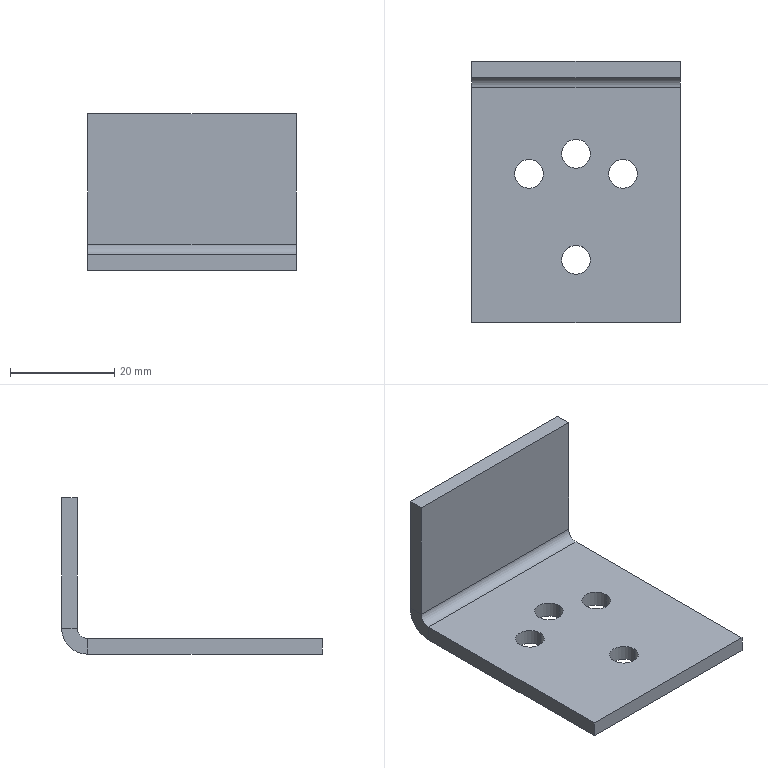Part | SolidWorks | features EdgeFlange 1, FlatPattern 1, HoleWzd 1, SMBaseFlange 1, SheetMetal 1 | 1 solid | 22 faces | box 40 x 50 x 30 mm | volume 8775 mm3 | plane 12 | cylinder 10 | commonest cylinder face diameters 5.5 x8 4 x1 10 x1
STEP:
#1=CARTESIAN_POINT('',(-11.75,3.5,-3.));
#2=VERTEX_POINT('',#1);
#3=CARTESIAN_POINT('',(-6.25,3.5,-3.));
#4=VERTEX_POINT('',#3);
#5=CARTESIAN_POINT('',(-9.,3.5,-3.));
#6=DIRECTION('',(0.,0.,1.));
#7=DIRECTION('',(1.,0.,0.));
#8=AXIS2_PLACEMENT_3D('',#5,#6,#7);
#9=CIRCLE('',#8,2.75);
#10=EDGE_CURVE('',#2,#4,#9,.T.);
#11=ORIENTED_EDGE('',*,*,#10,.F.);
#12=CARTESIAN_POINT('',(-11.75,3.5,0.));
#13=VERTEX_POINT('',#12);
#14=CARTESIAN_POINT('',(-11.75,3.5,0.));
#15=DIRECTION('',(0.,0.,1.));
#16=VECTOR('',#15,1000.);
#17=LINE('',#14,#16);
#18=EDGE_CURVE('',#2,#13,#17,.T.);
#19=ORIENTED_EDGE('',*,*,#18,.T.);
#20=CARTESIAN_POINT('',(-6.25,3.5,0.));
#21=VERTEX_POINT('',#20);
#22=CARTESIAN_POINT('',(-9.,3.5,0.));
#23=DIRECTION('',(0.,0.,1.));
#24=DIRECTION('',(1.,0.,0.));
#25=AXIS2_PLACEMENT_3D('',#22,#23,#24);
#26=CIRCLE('',#25,2.75);
#27=EDGE_CURVE('',#13,#21,#26,.T.);
#28=ORIENTED_EDGE('',*,*,#27,.T.);
#29=CARTESIAN_POINT('',(-6.25,3.5,0.));
#30=DIRECTION('',(0.,0.,1.));
#31=VECTOR('',#30,1000.);
#32=LINE('',#29,#31);
#33=EDGE_CURVE('',#4,#21,#32,.T.);
#34=ORIENTED_EDGE('',*,*,#33,.F.);
#35=EDGE_LOOP('',(#11,#19,#28,#34));
#36=FACE_OUTER_BOUND('',#35,.T.);
#37=CARTESIAN_POINT('',(-9.,3.5,0.));
#38=DIRECTION('',(0.,0.,1.));
#39=DIRECTION('',(1.,0.,0.));
#40=AXIS2_PLACEMENT_3D('',#37,#38,#39);
#41=CYLINDRICAL_SURFACE('',#40,2.75);
#42=ADVANCED_FACE('',(#36),#41,.F.);
#43=CARTESIAN_POINT('',(-2.75,7.35,-3.));
#44=VERTEX_POINT('',#43);
#45=CARTESIAN_POINT('',(2.75,7.35,-3.));
#46=VERTEX_POINT('',#45);
#47=CARTESIAN_POINT('',(0.,7.35,-3.));
#48=DIRECTION('',(0.,0.,1.));
#49=DIRECTION('',(1.,0.,0.));
#50=AXIS2_PLACEMENT_3D('',#47,#48,#49);
#51=CIRCLE('',#50,2.75);
#52=EDGE_CURVE('',#44,#46,#51,.T.);
#53=ORIENTED_EDGE('',*,*,#52,.F.);
#54=CARTESIAN_POINT('',(-2.75,7.35,0.));
#55=VERTEX_POINT('',#54);
#56=CARTESIAN_POINT('',(-2.75,7.35,0.));
#57=DIRECTION('',(0.,0.,1.));
#58=VECTOR('',#57,1000.);
#59=LINE('',#56,#58);
#60=EDGE_CURVE('',#44,#55,#59,.T.);
#61=ORIENTED_EDGE('',*,*,#60,.T.);
#62=CARTESIAN_POINT('',(2.75,7.35,0.));
#63=VERTEX_POINT('',#62);
#64=CARTESIAN_POINT('',(0.,7.35,0.));
#65=DIRECTION('',(0.,0.,1.));
#66=DIRECTION('',(1.,0.,0.));
#67=AXIS2_PLACEMENT_3D('',#64,#65,#66);
#68=CIRCLE('',#67,2.75);
#69=EDGE_CURVE('',#55,#63,#68,.T.);
#70=ORIENTED_EDGE('',*,*,#69,.T.);
#71=CARTESIAN_POINT('',(2.75,7.35,0.));
#72=DIRECTION('',(0.,0.,1.));
#73=VECTOR('',#72,1000.);
#74=LINE('',#71,#73);
#75=EDGE_CURVE('',#46,#63,#74,.T.);
#76=ORIENTED_EDGE('',*,*,#75,.F.);
#77=EDGE_LOOP('',(#53,#61,#70,#76));
#78=FACE_OUTER_BOUND('',#77,.T.);
#79=CARTESIAN_POINT('',(0.,7.35,0.));
#80=DIRECTION('',(0.,0.,1.));
#81=DIRECTION('',(1.,0.,0.));
#82=AXIS2_PLACEMENT_3D('',#79,#80,#81);
#83=CYLINDRICAL_SURFACE('',#82,2.75);
#84=ADVANCED_FACE('',(#78),#83,.F.);
#85=CARTESIAN_POINT('',(6.25,3.5,-3.));
#86=VERTEX_POINT('',#85);
#87=CARTESIAN_POINT('',(11.75,3.5,-3.));
#88=VERTEX_POINT('',#87);
#89=CARTESIAN_POINT('',(9.,3.5,-3.));
#90=DIRECTION('',(0.,0.,1.));
#91=DIRECTION('',(1.,0.,0.));
#92=AXIS2_PLACEMENT_3D('',#89,#90,#91);
#93=CIRCLE('',#92,2.75);
#94=EDGE_CURVE('',#86,#88,#93,.T.);
#95=ORIENTED_EDGE('',*,*,#94,.F.);
#96=CARTESIAN_POINT('',(6.25,3.5,0.));
#97=VERTEX_POINT('',#96);
#98=CARTESIAN_POINT('',(6.25,3.5,0.));
#99=DIRECTION('',(0.,0.,1.));
#100=VECTOR('',#99,1000.);
#101=LINE('',#98,#100);
#102=EDGE_CURVE('',#86,#97,#101,.T.);
#103=ORIENTED_EDGE('',*,*,#102,.T.);
#104=CARTESIAN_POINT('',(11.75,3.5,0.));
#105=VERTEX_POINT('',#104);
#106=CARTESIAN_POINT('',(9.,3.5,0.));
#107=DIRECTION('',(0.,0.,1.));
#108=DIRECTION('',(1.,0.,0.));
#109=AXIS2_PLACEMENT_3D('',#106,#107,#108);
#110=CIRCLE('',#109,2.75);
#111=EDGE_CURVE('',#97,#105,#110,.T.);
#112=ORIENTED_EDGE('',*,*,#111,.T.);
#113=CARTESIAN_POINT('',(11.75,3.5,0.));
#114=DIRECTION('',(0.,0.,1.));
#115=VECTOR('',#114,1000.);
#116=LINE('',#113,#115);
#117=EDGE_CURVE('',#88,#105,#116,.T.);
#118=ORIENTED_EDGE('',*,*,#117,.F.);
#119=EDGE_LOOP('',(#95,#103,#112,#118));
#120=FACE_OUTER_BOUND('',#119,.T.);
#121=CARTESIAN_POINT('',(9.,3.5,0.));
#122=DIRECTION('',(0.,0.,1.));
#123=DIRECTION('',(1.,0.,0.));
#124=AXIS2_PLACEMENT_3D('',#121,#122,#123);
#125=CYLINDRICAL_SURFACE('',#124,2.75);
#126=ADVANCED_FACE('',(#120),#125,.F.);
#127=CARTESIAN_POINT('',(-2.75,-12.988,-3.));
#128=VERTEX_POINT('',#127);
#129=CARTESIAN_POINT('',(2.75,-12.988,-3.));
#130=VERTEX_POINT('',#129);
#131=CARTESIAN_POINT('',(-0.000000118,-12.988,-3.));
#132=DIRECTION('',(0.,0.,1.));
#133=DIRECTION('',(1.,0.,0.));
#134=AXIS2_PLACEMENT_3D('',#131,#132,#133);
#135=CIRCLE('',#134,2.75);
#136=EDGE_CURVE('',#128,#130,#135,.T.);
#137=ORIENTED_EDGE('',*,*,#136,.F.);
#138=CARTESIAN_POINT('',(-2.75,-12.988,0.));
#139=VERTEX_POINT('',#138);
#140=CARTESIAN_POINT('',(-2.75,-12.988,0.));
#141=DIRECTION('',(0.,0.,1.));
#142=VECTOR('',#141,1000.);
#143=LINE('',#140,#142);
#144=EDGE_CURVE('',#128,#139,#143,.T.);
#145=ORIENTED_EDGE('',*,*,#144,.T.);
#146=CARTESIAN_POINT('',(2.75,-12.988,0.));
#147=VERTEX_POINT('',#146);
#148=CARTESIAN_POINT('',(-0.000000118,-12.988,0.));
#149=DIRECTION('',(0.,0.,1.));
#150=DIRECTION('',(1.,0.,0.));
#151=AXIS2_PLACEMENT_3D('',#148,#149,#150);
#152=CIRCLE('',#151,2.75);
#153=EDGE_CURVE('',#139,#147,#152,.T.);
#154=ORIENTED_EDGE('',*,*,#153,.T.);
#155=CARTESIAN_POINT('',(2.75,-12.988,0.));
#156=DIRECTION('',(0.,0.,1.));
#157=VECTOR('',#156,1000.);
#158=LINE('',#155,#157);
#159=EDGE_CURVE('',#130,#147,#158,.T.);
#160=ORIENTED_EDGE('',*,*,#159,.F.);
#161=EDGE_LOOP('',(#137,#145,#154,#160));
#162=FACE_OUTER_BOUND('',#161,.T.);
#163=CARTESIAN_POINT('',(-0.000000118,-12.988,0.));
#164=DIRECTION('',(0.,0.,1.));
#165=DIRECTION('',(1.,0.,0.));
#166=AXIS2_PLACEMENT_3D('',#163,#164,#165);
#167=CYLINDRICAL_SURFACE('',#166,2.75);
#168=ADVANCED_FACE('',(#162),#167,.F.);
#169=CARTESIAN_POINT('',(-20.,20.,0.));
#170=VERTEX_POINT('',#169);
#171=CARTESIAN_POINT('',(-20.,-25.,0.));
#172=VERTEX_POINT('',#171);
#173=CARTESIAN_POINT('',(-20.,-25.,0.));
#174=DIRECTION('',(0.,-1.,0.));
#175=VECTOR('',#174,1000.);
#176=LINE('',#173,#175);
#177=EDGE_CURVE('',#170,#172,#176,.T.);
#178=ORIENTED_EDGE('',*,*,#177,.F.);
#179=CARTESIAN_POINT('',(-20.,20.,-3.));
#180=VERTEX_POINT('',#179);
#181=CARTESIAN_POINT('',(-20.,20.,0.));
#182=DIRECTION('',(0.,0.,-1.));
#183=VECTOR('',#182,1000.);
#184=LINE('',#181,#183);
#185=EDGE_CURVE('',#170,#180,#184,.T.);
#186=ORIENTED_EDGE('',*,*,#185,.T.);
#187=CARTESIAN_POINT('',(-20.,-25.,-3.));
#188=VERTEX_POINT('',#187);
#189=CARTESIAN_POINT('',(-20.,-25.,-3.));
#190=DIRECTION('',(0.,-1.,0.));
#191=VECTOR('',#190,1000.);
#192=LINE('',#189,#191);
#193=EDGE_CURVE('',#180,#188,#192,.T.);
#194=ORIENTED_EDGE('',*,*,#193,.T.);
#195=CARTESIAN_POINT('',(-20.,-25.,-3.));
#196=DIRECTION('',(0.,0.,1.));
#197=VECTOR('',#196,1000.);
#198=LINE('',#195,#197);
#199=EDGE_CURVE('',#188,#172,#198,.T.);
#200=ORIENTED_EDGE('',*,*,#199,.T.);
#201=EDGE_LOOP('',(#178,#186,#194,#200));
#202=FACE_OUTER_BOUND('',#201,.T.);
#203=CARTESIAN_POINT('',(-20.,-25.,-3.));
#204=DIRECTION('',(-1.,0.,0.));
#205=DIRECTION('',(0.,0.,1.));
#206=AXIS2_PLACEMENT_3D('',#203,#204,#205);
#207=PLANE('',#206);
#208=ADVANCED_FACE('',(#202),#207,.T.);
#209=CARTESIAN_POINT('',(-9.,3.5,-3.));
#210=DIRECTION('',(0.,0.,1.));
#211=DIRECTION('',(1.,0.,0.));
#212=AXIS2_PLACEMENT_3D('',#209,#210,#211);
#213=CIRCLE('',#212,2.75);
#214=EDGE_CURVE('',#4,#2,#213,.T.);
#215=ORIENTED_EDGE('',*,*,#214,.T.);
#216=ORIENTED_EDGE('',*,*,#10,.T.);
#217=EDGE_LOOP('',(#215,#216));
#218=FACE_BOUND('',#217,.T.);
#219=CARTESIAN_POINT('',(0.,7.35,-3.));
#220=DIRECTION('',(0.,0.,1.));
#221=DIRECTION('',(1.,0.,0.));
#222=AXIS2_PLACEMENT_3D('',#219,#220,#221);
#223=CIRCLE('',#222,2.75);
#224=EDGE_CURVE('',#46,#44,#223,.T.);
#225=ORIENTED_EDGE('',*,*,#224,.T.);
#226=ORIENTED_EDGE('',*,*,#52,.T.);
#227=EDGE_LOOP('',(#225,#226));
#228=FACE_BOUND('',#227,.T.);
#229=CARTESIAN_POINT('',(9.,3.5,-3.));
#230=DIRECTION('',(0.,0.,1.));
#231=DIRECTION('',(1.,0.,0.));
#232=AXIS2_PLACEMENT_3D('',#229,#230,#231);
#233=CIRCLE('',#232,2.75);
#234=EDGE_CURVE('',#88,#86,#233,.T.);
#235=ORIENTED_EDGE('',*,*,#234,.T.);
#236=ORIENTED_EDGE('',*,*,#94,.T.);
#237=EDGE_LOOP('',(#235,#236));
#238=FACE_BOUND('',#237,.T.);
#239=CARTESIAN_POINT('',(-0.000000118,-12.988,-3.));
#240=DIRECTION('',(0.,0.,1.));
#241=DIRECTION('',(1.,0.,0.));
#242=AXIS2_PLACEMENT_3D('',#239,#240,#241);
#243=CIRCLE('',#242,2.75);
#244=EDGE_CURVE('',#130,#128,#243,.T.);
#245=ORIENTED_EDGE('',*,*,#244,.T.);
#246=ORIENTED_EDGE('',*,*,#136,.T.);
#247=EDGE_LOOP('',(#245,#246));
#248=FACE_BOUND('',#247,.T.);
#249=ORIENTED_EDGE('',*,*,#193,.F.);
#250=CARTESIAN_POINT('',(20.,20.,-3.));
#251=VERTEX_POINT('',#250);
#252=CARTESIAN_POINT('',(-20.,20.,-3.));
#253=DIRECTION('',(1.,0.,0.));
#254=VECTOR('',#253,1000.);
#255=LINE('',#252,#254);
#256=EDGE_CURVE('',#180,#251,#255,.T.);
#257=ORIENTED_EDGE('',*,*,#256,.T.);
#258=CARTESIAN_POINT('',(20.,-25.,-3.));
#259=VERTEX_POINT('',#258);
#260=CARTESIAN_POINT('',(20.,-25.,-3.));
#261=DIRECTION('',(0.,1.,0.));
#262=VECTOR('',#261,1000.);
#263=LINE('',#260,#262);
#264=EDGE_CURVE('',#259,#251,#263,.T.);
#265=ORIENTED_EDGE('',*,*,#264,.F.);
#266=CARTESIAN_POINT('',(-20.,-25.,-3.));
#267=DIRECTION('',(1.,0.,0.));
#268=VECTOR('',#267,1000.);
#269=LINE('',#266,#268);
#270=EDGE_CURVE('',#188,#259,#269,.T.);
#271=ORIENTED_EDGE('',*,*,#270,.F.);
#272=EDGE_LOOP('',(#249,#257,#265,#271));
#273=FACE_OUTER_BOUND('',#272,.T.);
#274=CARTESIAN_POINT('',(0.,0.,-3.));
#275=DIRECTION('',(0.,0.,-1.));
#276=DIRECTION('',(-1.,0.,0.));
#277=AXIS2_PLACEMENT_3D('',#274,#275,#276);
#278=PLANE('',#277);
#279=ADVANCED_FACE('',(#218,#228,#238,#248,#273),#278,.T.);
#280=CARTESIAN_POINT('',(-9.,3.5,0.));
#281=DIRECTION('',(0.,0.,1.));
#282=DIRECTION('',(1.,0.,0.));
#283=AXIS2_PLACEMENT_3D('',#280,#281,#282);
#284=CIRCLE('',#283,2.75);
#285=EDGE_CURVE('',#21,#13,#284,.T.);
#286=ORIENTED_EDGE('',*,*,#285,.F.);
#287=ORIENTED_EDGE('',*,*,#27,.F.);
#288=EDGE_LOOP('',(#286,#287));
#289=FACE_BOUND('',#288,.T.);
#290=CARTESIAN_POINT('',(0.,7.35,0.));
#291=DIRECTION('',(0.,0.,1.));
#292=DIRECTION('',(1.,0.,0.));
#293=AXIS2_PLACEMENT_3D('',#290,#291,#292);
#294=CIRCLE('',#293,2.75);
#295=EDGE_CURVE('',#63,#55,#294,.T.);
#296=ORIENTED_EDGE('',*,*,#295,.F.);
#297=ORIENTED_EDGE('',*,*,#69,.F.);
#298=EDGE_LOOP('',(#296,#297));
#299=FACE_BOUND('',#298,.T.);
#300=CARTESIAN_POINT('',(9.,3.5,0.));
#301=DIRECTION('',(0.,0.,1.));
#302=DIRECTION('',(1.,0.,0.));
#303=AXIS2_PLACEMENT_3D('',#300,#301,#302);
#304=CIRCLE('',#303,2.75);
#305=EDGE_CURVE('',#105,#97,#304,.T.);
#306=ORIENTED_EDGE('',*,*,#305,.F.);
#307=ORIENTED_EDGE('',*,*,#111,.F.);
#308=EDGE_LOOP('',(#306,#307));
#309=FACE_BOUND('',#308,.T.);
#310=CARTESIAN_POINT('',(-0.000000118,-12.988,0.));
#311=DIRECTION('',(0.,0.,1.));
#312=DIRECTION('',(1.,0.,0.));
#313=AXIS2_PLACEMENT_3D('',#310,#311,#312);
#314=CIRCLE('',#313,2.75);
#315=EDGE_CURVE('',#147,#139,#314,.T.);
#316=ORIENTED_EDGE('',*,*,#315,.F.);
#317=ORIENTED_EDGE('',*,*,#153,.F.);
#318=EDGE_LOOP('',(#316,#317));
#319=FACE_BOUND('',#318,.T.);
#320=CARTESIAN_POINT('',(20.,20.,0.));
#321=VERTEX_POINT('',#320);
#322=CARTESIAN_POINT('',(-20.,20.,0.));
#323=DIRECTION('',(1.,0.,0.));
#324=VECTOR('',#323,1000.);
#325=LINE('',#322,#324);
#326=EDGE_CURVE('',#170,#321,#325,.T.);
#327=ORIENTED_EDGE('',*,*,#326,.F.);
#328=ORIENTED_EDGE('',*,*,#177,.T.);
#329=CARTESIAN_POINT('',(20.,-25.,0.));
#330=VERTEX_POINT('',#329);
#331=CARTESIAN_POINT('',(-20.,-25.,0.));
#332=DIRECTION('',(1.,0.,0.));
#333=VECTOR('',#332,1000.);
#334=LINE('',#331,#333);
#335=EDGE_CURVE('',#172,#330,#334,.T.);
#336=ORIENTED_EDGE('',*,*,#335,.T.);
#337=CARTESIAN_POINT('',(20.,-25.,0.));
#338=DIRECTION('',(0.,1.,0.));
#339=VECTOR('',#338,1000.);
#340=LINE('',#337,#339);
#341=EDGE_CURVE('',#330,#321,#340,.T.);
#342=ORIENTED_EDGE('',*,*,#341,.T.);
#343=EDGE_LOOP('',(#327,#328,#336,#342));
#344=FACE_OUTER_BOUND('',#343,.T.);
#345=CARTESIAN_POINT('',(0.,0.,0.));
#346=DIRECTION('',(0.,0.,-1.));
#347=DIRECTION('',(-1.,0.,0.));
#348=AXIS2_PLACEMENT_3D('',#345,#346,#347);
#349=PLANE('',#348);
#350=ADVANCED_FACE('',(#289,#299,#309,#319,#344),#349,.F.);
#351=CARTESIAN_POINT('',(20.,20.,0.));
#352=DIRECTION('',(0.,0.,-1.));
#353=VECTOR('',#352,1000.);
#354=LINE('',#351,#353);
#355=EDGE_CURVE('',#321,#251,#354,.T.);
#356=ORIENTED_EDGE('',*,*,#355,.F.);
#357=ORIENTED_EDGE('',*,*,#341,.F.);
#358=CARTESIAN_POINT('',(20.,-25.,-3.));
#359=DIRECTION('',(0.,0.,1.));
#360=VECTOR('',#359,1000.);
#361=LINE('',#358,#360);
#362=EDGE_CURVE('',#259,#330,#361,.T.);
#363=ORIENTED_EDGE('',*,*,#362,.F.);
#364=ORIENTED_EDGE('',*,*,#264,.T.);
#365=EDGE_LOOP('',(#356,#357,#363,#364));
#366=FACE_OUTER_BOUND('',#365,.T.);
#367=CARTESIAN_POINT('',(20.,-25.,-3.));
#368=DIRECTION('',(1.,0.,0.));
#369=DIRECTION('',(0.,0.,-1.));
#370=AXIS2_PLACEMENT_3D('',#367,#368,#369);
#371=PLANE('',#370);
#372=ADVANCED_FACE('',(#366),#371,.T.);
#373=ORIENTED_EDGE('',*,*,#335,.F.);
#374=ORIENTED_EDGE('',*,*,#199,.F.);
#375=ORIENTED_EDGE('',*,*,#270,.T.);
#376=ORIENTED_EDGE('',*,*,#362,.T.);
#377=EDGE_LOOP('',(#373,#374,#375,#376));
#378=FACE_OUTER_BOUND('',#377,.T.);
#379=CARTESIAN_POINT('',(-20.,-25.,-3.));
#380=DIRECTION('',(0.,-1.,0.));
#381=DIRECTION('',(0.,0.,-1.));
#382=AXIS2_PLACEMENT_3D('',#379,#380,#381);
#383=PLANE('',#382);
#384=ADVANCED_FACE('',(#378),#383,.T.);
#385=CARTESIAN_POINT('',(20.,22.,2.));
#386=VERTEX_POINT('',#385);
#387=CARTESIAN_POINT('',(20.,25.,2.));
#388=VERTEX_POINT('',#387);
#389=CARTESIAN_POINT('',(20.,25.,2.));
#390=DIRECTION('',(0.,1.,0.));
#391=VECTOR('',#390,1000.);
#392=LINE('',#389,#391);
#393=EDGE_CURVE('',#386,#388,#392,.T.);
#394=ORIENTED_EDGE('',*,*,#393,.F.);
#395=CARTESIAN_POINT('',(20.,20.,2.));
#396=DIRECTION('',(1.,0.,0.));
#397=DIRECTION('',(0.,0.,1.));
#398=AXIS2_PLACEMENT_3D('',#395,#396,#397);
#399=CIRCLE('',#398,2.);
#400=EDGE_CURVE('',#321,#386,#399,.T.);
#401=ORIENTED_EDGE('',*,*,#400,.F.);
#402=ORIENTED_EDGE('',*,*,#355,.T.);
#403=CARTESIAN_POINT('',(20.,20.,2.));
#404=DIRECTION('',(1.,0.,0.));
#405=DIRECTION('',(0.,0.,1.));
#406=AXIS2_PLACEMENT_3D('',#403,#404,#405);
#407=CIRCLE('',#406,5.);
#408=EDGE_CURVE('',#251,#388,#407,.T.);
#409=ORIENTED_EDGE('',*,*,#408,.T.);
#410=EDGE_LOOP('',(#394,#401,#402,#409));
#411=FACE_OUTER_BOUND('',#410,.T.);
#412=CARTESIAN_POINT('',(20.,20.,2.));
#413=DIRECTION('',(1.,0.,0.));
#414=DIRECTION('',(0.,0.,-1.));
#415=AXIS2_PLACEMENT_3D('',#412,#413,#414);
#416=PLANE('',#415);
#417=ADVANCED_FACE('',(#411),#416,.T.);
#418=CARTESIAN_POINT('',(-20.,22.,2.));
#419=VERTEX_POINT('',#418);
#420=CARTESIAN_POINT('',(-20.,20.,2.));
#421=DIRECTION('',(-1.,0.,0.));
#422=DIRECTION('',(0.,0.,1.));
#423=AXIS2_PLACEMENT_3D('',#420,#421,#422);
#424=CIRCLE('',#423,2.);
#425=EDGE_CURVE('',#419,#170,#424,.T.);
#426=ORIENTED_EDGE('',*,*,#425,.F.);
#427=CARTESIAN_POINT('',(-20.,25.,2.));
#428=VERTEX_POINT('',#427);
#429=CARTESIAN_POINT('',(-20.,22.,2.));
#430=DIRECTION('',(0.,1.,0.));
#431=VECTOR('',#430,1000.);
#432=LINE('',#429,#431);
#433=EDGE_CURVE('',#419,#428,#432,.T.);
#434=ORIENTED_EDGE('',*,*,#433,.T.);
#435=CARTESIAN_POINT('',(-20.,20.,2.));
#436=DIRECTION('',(-1.,0.,0.));
#437=DIRECTION('',(0.,0.,1.));
#438=AXIS2_PLACEMENT_3D('',#435,#436,#437);
#439=CIRCLE('',#438,5.);
#440=EDGE_CURVE('',#428,#180,#439,.T.);
#441=ORIENTED_EDGE('',*,*,#440,.T.);
#442=ORIENTED_EDGE('',*,*,#185,.F.);
#443=EDGE_LOOP('',(#426,#434,#441,#442));
#444=FACE_OUTER_BOUND('',#443,.T.);
#445=CARTESIAN_POINT('',(-20.,20.,2.));
#446=DIRECTION('',(1.,0.,0.));
#447=DIRECTION('',(0.,0.,-1.));
#448=AXIS2_PLACEMENT_3D('',#445,#446,#447);
#449=PLANE('',#448);
#450=ADVANCED_FACE('',(#444),#449,.F.);
#451=ORIENTED_EDGE('',*,*,#256,.F.);
#452=ORIENTED_EDGE('',*,*,#440,.F.);
#453=CARTESIAN_POINT('',(20.,25.,2.));
#454=DIRECTION('',(1.,0.,0.));
#455=VECTOR('',#454,1000.);
#456=LINE('',#453,#455);
#457=EDGE_CURVE('',#428,#388,#456,.T.);
#458=ORIENTED_EDGE('',*,*,#457,.T.);
#459=ORIENTED_EDGE('',*,*,#408,.F.);
#460=EDGE_LOOP('',(#451,#452,#458,#459));
#461=FACE_OUTER_BOUND('',#460,.T.);
#462=CARTESIAN_POINT('',(-20.,20.,2.));
#463=DIRECTION('',(-1.,0.,0.));
#464=DIRECTION('',(0.,1.,0.));
#465=AXIS2_PLACEMENT_3D('',#462,#463,#464);
#466=CYLINDRICAL_SURFACE('',#465,5.);
#467=ADVANCED_FACE('',(#461),#466,.T.);
#468=ORIENTED_EDGE('',*,*,#326,.T.);
#469=ORIENTED_EDGE('',*,*,#400,.T.);
#470=CARTESIAN_POINT('',(20.,22.,2.));
#471=DIRECTION('',(-1.,0.,0.));
#472=VECTOR('',#471,1000.);
#473=LINE('',#470,#472);
#474=EDGE_CURVE('',#386,#419,#473,.T.);
#475=ORIENTED_EDGE('',*,*,#474,.T.);
#476=ORIENTED_EDGE('',*,*,#425,.T.);
#477=EDGE_LOOP('',(#468,#469,#475,#476));
#478=FACE_OUTER_BOUND('',#477,.T.);
#479=CARTESIAN_POINT('',(-20.,20.,2.));
#480=DIRECTION('',(-1.,0.,0.));
#481=DIRECTION('',(0.,1.,0.));
#482=AXIS2_PLACEMENT_3D('',#479,#480,#481);
#483=CYLINDRICAL_SURFACE('',#482,2.);
#484=ADVANCED_FACE('',(#478),#483,.F.);
#485=ORIENTED_EDGE('',*,*,#393,.T.);
#486=CARTESIAN_POINT('',(20.,25.,27.));
#487=VERTEX_POINT('',#486);
#488=CARTESIAN_POINT('',(20.,25.,0.));
#489=DIRECTION('',(0.,0.,-1.));
#490=VECTOR('',#489,1000.);
#491=LINE('',#488,#490);
#492=EDGE_CURVE('',#487,#388,#491,.T.);
#493=ORIENTED_EDGE('',*,*,#492,.F.);
#494=CARTESIAN_POINT('',(20.,22.,27.));
#495=VERTEX_POINT('',#494);
#496=CARTESIAN_POINT('',(20.,25.,27.));
#497=DIRECTION('',(0.,-1.,0.));
#498=VECTOR('',#497,1000.);
#499=LINE('',#496,#498);
#500=EDGE_CURVE('',#487,#495,#499,.T.);
#501=ORIENTED_EDGE('',*,*,#500,.T.);
#502=CARTESIAN_POINT('',(20.,22.,0.));
#503=DIRECTION('',(0.,0.,-1.));
#504=VECTOR('',#503,1000.);
#505=LINE('',#502,#504);
#506=EDGE_CURVE('',#495,#386,#505,.T.);
#507=ORIENTED_EDGE('',*,*,#506,.T.);
#508=EDGE_LOOP('',(#485,#493,#501,#507));
#509=FACE_OUTER_BOUND('',#508,.T.);
#510=CARTESIAN_POINT('',(20.,25.,0.));
#511=DIRECTION('',(-1.,0.,0.));
#512=DIRECTION('',(0.,0.,1.));
#513=AXIS2_PLACEMENT_3D('',#510,#511,#512);
#514=PLANE('',#513);
#515=ADVANCED_FACE('',(#509),#514,.F.);
#516=ORIENTED_EDGE('',*,*,#433,.F.);
#517=CARTESIAN_POINT('',(-20.,22.,27.));
#518=VERTEX_POINT('',#517);
#519=CARTESIAN_POINT('',(-20.,22.,27.));
#520=DIRECTION('',(0.,0.,1.));
#521=VECTOR('',#520,1000.);
#522=LINE('',#519,#521);
#523=EDGE_CURVE('',#419,#518,#522,.T.);
#524=ORIENTED_EDGE('',*,*,#523,.T.);
#525=CARTESIAN_POINT('',(-20.,25.,27.));
#526=VERTEX_POINT('',#525);
#527=CARTESIAN_POINT('',(-20.,25.,27.));
#528=DIRECTION('',(0.,-1.,0.));
#529=VECTOR('',#528,1000.);
#530=LINE('',#527,#529);
#531=EDGE_CURVE('',#526,#518,#530,.T.);
#532=ORIENTED_EDGE('',*,*,#531,.F.);
#533=CARTESIAN_POINT('',(-20.,25.,0.));
#534=DIRECTION('',(0.,0.,1.));
#535=VECTOR('',#534,1000.);
#536=LINE('',#533,#535);
#537=EDGE_CURVE('',#428,#526,#536,.T.);
#538=ORIENTED_EDGE('',*,*,#537,.F.);
#539=EDGE_LOOP('',(#516,#524,#532,#538));
#540=FACE_OUTER_BOUND('',#539,.T.);
#541=CARTESIAN_POINT('',(-20.,25.,27.));
#542=DIRECTION('',(1.,0.,0.));
#543=DIRECTION('',(0.,0.,-1.));
#544=AXIS2_PLACEMENT_3D('',#541,#542,#543);
#545=PLANE('',#544);
#546=ADVANCED_FACE('',(#540),#545,.F.);
#547=ORIENTED_EDGE('',*,*,#457,.F.);
#548=ORIENTED_EDGE('',*,*,#537,.T.);
#549=CARTESIAN_POINT('',(0.,25.,27.));
#550=DIRECTION('',(1.,0.,0.));
#551=VECTOR('',#550,1000.);
#552=LINE('',#549,#551);
#553=EDGE_CURVE('',#526,#487,#552,.T.);
#554=ORIENTED_EDGE('',*,*,#553,.T.);
#555=ORIENTED_EDGE('',*,*,#492,.T.);
#556=EDGE_LOOP('',(#547,#548,#554,#555));
#557=FACE_OUTER_BOUND('',#556,.T.);
#558=CARTESIAN_POINT('',(0.,25.,0.));
#559=DIRECTION('',(0.,-1.,0.));
#560=DIRECTION('',(0.,0.,-1.));
#561=AXIS2_PLACEMENT_3D('',#558,#559,#560);
#562=PLANE('',#561);
#563=ADVANCED_FACE('',(#557),#562,.F.);
#564=ORIENTED_EDGE('',*,*,#523,.F.);
#565=ORIENTED_EDGE('',*,*,#474,.F.);
#566=ORIENTED_EDGE('',*,*,#506,.F.);
#567=CARTESIAN_POINT('',(20.,22.,27.));
#568=DIRECTION('',(1.,0.,0.));
#569=VECTOR('',#568,1000.);
#570=LINE('',#567,#569);
#571=EDGE_CURVE('',#518,#495,#570,.T.);
#572=ORIENTED_EDGE('',*,*,#571,.F.);
#573=EDGE_LOOP('',(#564,#565,#566,#572));
#574=FACE_OUTER_BOUND('',#573,.T.);
#575=CARTESIAN_POINT('',(0.,22.,0.));
#576=DIRECTION('',(0.,-1.,0.));
#577=DIRECTION('',(0.,0.,-1.));
#578=AXIS2_PLACEMENT_3D('',#575,#576,#577);
#579=PLANE('',#578);
#580=ADVANCED_FACE('',(#574),#579,.T.);
#581=ORIENTED_EDGE('',*,*,#571,.T.);
#582=ORIENTED_EDGE('',*,*,#500,.F.);
#583=ORIENTED_EDGE('',*,*,#553,.F.);
#584=ORIENTED_EDGE('',*,*,#531,.T.);
#585=EDGE_LOOP('',(#581,#582,#583,#584));
#586=FACE_OUTER_BOUND('',#585,.T.);
#587=CARTESIAN_POINT('',(20.,25.,27.));
#588=DIRECTION('',(0.,0.,-1.));
#589=DIRECTION('',(0.,1.,0.));
#590=AXIS2_PLACEMENT_3D('',#587,#588,#589);
#591=PLANE('',#590);
#592=ADVANCED_FACE('',(#586),#591,.F.);
#593=ORIENTED_EDGE('',*,*,#144,.F.);
#594=ORIENTED_EDGE('',*,*,#244,.F.);
#595=ORIENTED_EDGE('',*,*,#159,.T.);
#596=ORIENTED_EDGE('',*,*,#315,.T.);
#597=EDGE_LOOP('',(#593,#594,#595,#596));
#598=FACE_OUTER_BOUND('',#597,.T.);
#599=CARTESIAN_POINT('',(-0.000000118,-12.988,0.));
#600=DIRECTION('',(0.,0.,1.));
#601=DIRECTION('',(1.,0.,0.));
#602=AXIS2_PLACEMENT_3D('',#599,#600,#601);
#603=CYLINDRICAL_SURFACE('',#602,2.75);
#604=ADVANCED_FACE('',(#598),#603,.F.);
#605=ORIENTED_EDGE('',*,*,#102,.F.);
#606=ORIENTED_EDGE('',*,*,#234,.F.);
#607=ORIENTED_EDGE('',*,*,#117,.T.);
#608=ORIENTED_EDGE('',*,*,#305,.T.);
#609=EDGE_LOOP('',(#605,#606,#607,#608));
#610=FACE_OUTER_BOUND('',#609,.T.);
#611=CARTESIAN_POINT('',(9.,3.5,0.));
#612=DIRECTION('',(0.,0.,1.));
#613=DIRECTION('',(1.,0.,0.));
#614=AXIS2_PLACEMENT_3D('',#611,#612,#613);
#615=CYLINDRICAL_SURFACE('',#614,2.75);
#616=ADVANCED_FACE('',(#610),#615,.F.);
#617=ORIENTED_EDGE('',*,*,#60,.F.);
#618=ORIENTED_EDGE('',*,*,#224,.F.);
#619=ORIENTED_EDGE('',*,*,#75,.T.);
#620=ORIENTED_EDGE('',*,*,#295,.T.);
#621=EDGE_LOOP('',(#617,#618,#619,#620));
#622=FACE_OUTER_BOUND('',#621,.T.);
#623=CARTESIAN_POINT('',(0.,7.35,0.));
#624=DIRECTION('',(0.,0.,1.));
#625=DIRECTION('',(1.,0.,0.));
#626=AXIS2_PLACEMENT_3D('',#623,#624,#625);
#627=CYLINDRICAL_SURFACE('',#626,2.75);
#628=ADVANCED_FACE('',(#622),#627,.F.);
#629=ORIENTED_EDGE('',*,*,#18,.F.);
#630=ORIENTED_EDGE('',*,*,#214,.F.);
#631=ORIENTED_EDGE('',*,*,#33,.T.);
#632=ORIENTED_EDGE('',*,*,#285,.T.);
#633=EDGE_LOOP('',(#629,#630,#631,#632));
#634=FACE_OUTER_BOUND('',#633,.T.);
#635=CARTESIAN_POINT('',(-9.,3.5,0.));
#636=DIRECTION('',(0.,0.,1.));
#637=DIRECTION('',(1.,0.,0.));
#638=AXIS2_PLACEMENT_3D('',#635,#636,#637);
#639=CYLINDRICAL_SURFACE('',#638,2.75);
#640=ADVANCED_FACE('',(#634),#639,.F.);
#641=CLOSED_SHELL('',(#42,#84,#126,#168,#208,#279,#350,#372,#384,#417,#450,#467,#484,#515,#546,#563,#580,#592,#604,#616,#628,#640));
#642=MANIFOLD_SOLID_BREP('',#641);
#643=CARTESIAN_POINT('',(0.,0.,0.));
#644=DIRECTION('',(0.,0.,1.));
#645=DIRECTION('',(1.,0.,0.));
#646=AXIS2_PLACEMENT_3D('',#643,#644,#645);
#647=(LENGTH_UNIT()NAMED_UNIT(*)SI_UNIT(.MILLI.,.METRE.));
#648=UNCERTAINTY_MEASURE_WITH_UNIT(LENGTH_MEASURE(0.00001),#647,'','');
#649=(NAMED_UNIT(*)PLANE_ANGLE_UNIT()SI_UNIT($,.RADIAN.));
#650=(NAMED_UNIT(*)SI_UNIT($,.STERADIAN.)SOLID_ANGLE_UNIT());
#651=(GEOMETRIC_REPRESENTATION_CONTEXT(3)GLOBAL_UNCERTAINTY_ASSIGNED_CONTEXT((#648))GLOBAL_UNIT_ASSIGNED_CONTEXT((#647,#649,#650))REPRESENTATION_CONTEXT('',''));
#652=ADVANCED_BREP_SHAPE_REPRESENTATION('',(#642,#646),#651);